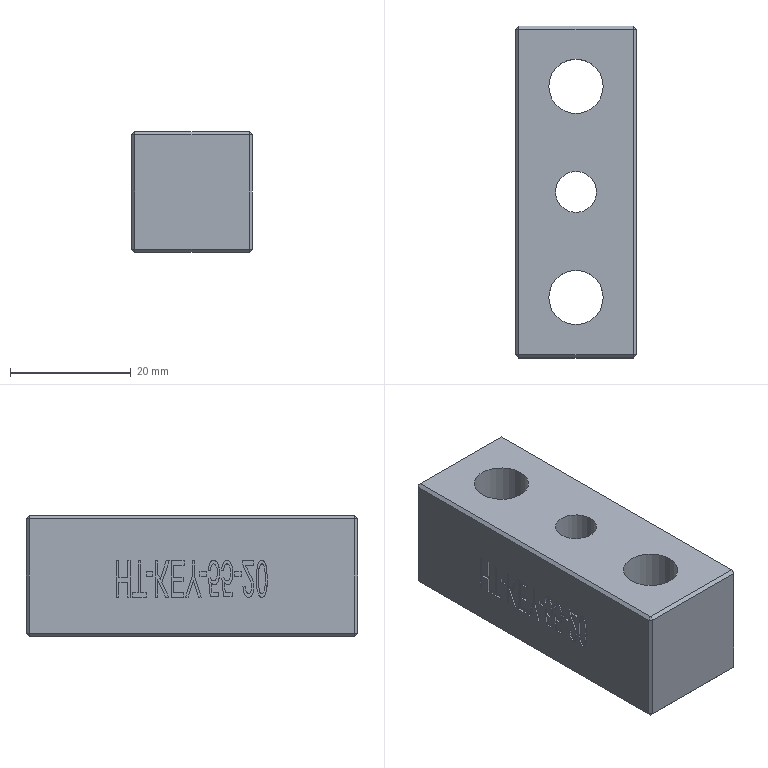Part | NX | features J 2 | 1 solid | 165 faces | box 20 x 55 x 20 mm | volume 16644 mm3 | plane 125 | spline 34 | cylinder 6 | commonest cylinder face diameters 9 x3 14 x2 6.8 x1